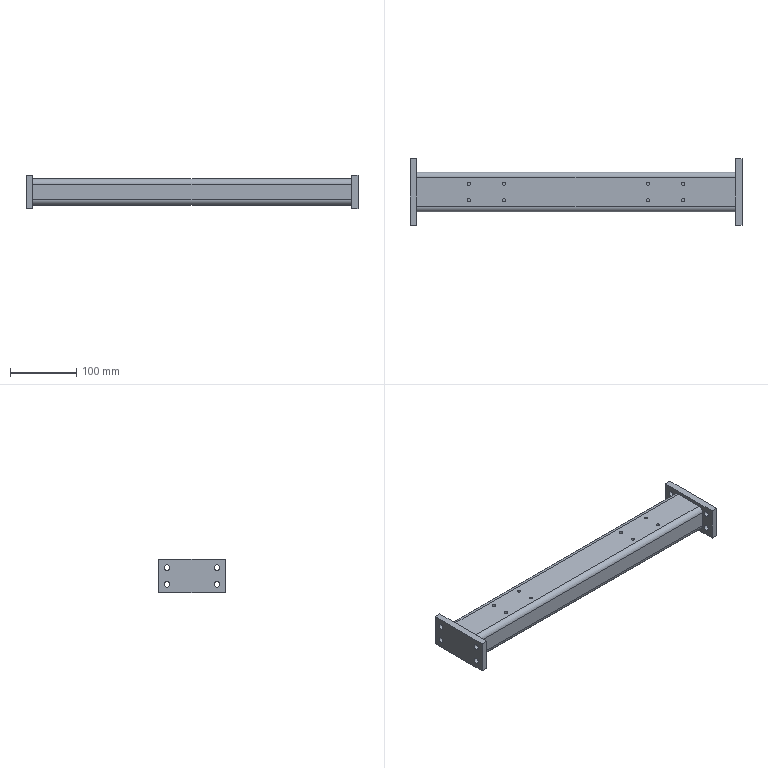Part | STEP file | PN_0007_support beam_default_machined_ | 3 solids | 82 faces | box 500 x 100 x 50 mm | volume 427549 mm3 | cylinder 60 | plane 22 | commonest cylinder face diameters 5 x36 8.5 x16 8 x4 16 x4